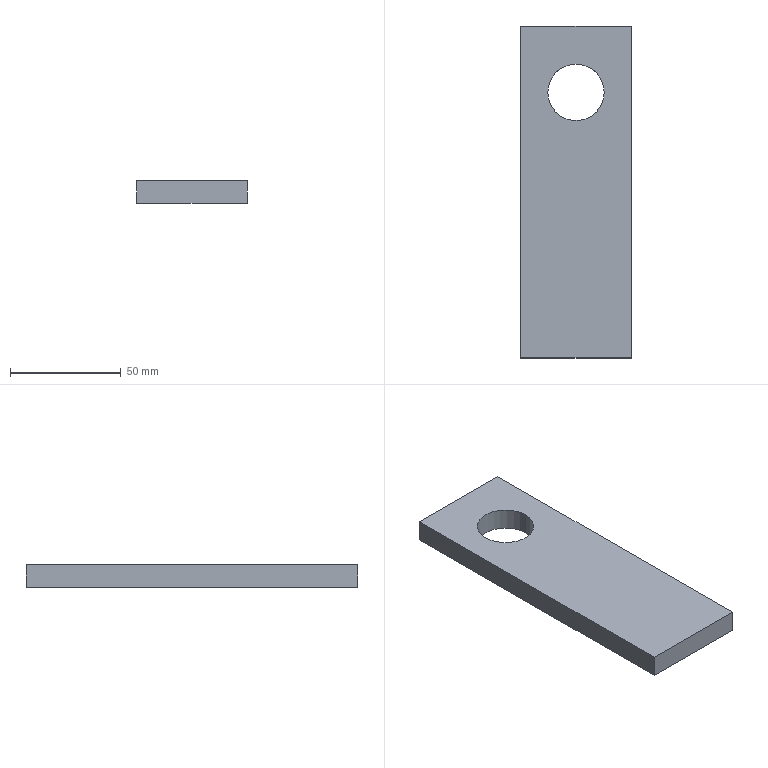Part | SolidWorks | features Extrusion 1, ICE 1 | 1 solid | 8 faces | box 50 x 150 x 10 mm | volume 69893 mm3 | plane 6 | cylinder 2 | commonest cylinder face diameters 25.5 x2
STEP:
#1=CARTESIAN_POINT('',(-12.75,45.,-5.));
#2=VERTEX_POINT('',#1);
#3=CARTESIAN_POINT('',(12.75,45.,-5.));
#4=VERTEX_POINT('',#3);
#5=CARTESIAN_POINT('',(0.,45.,-5.));
#6=DIRECTION('',(0.,0.,1.));
#7=DIRECTION('',(-1.,0.,0.));
#8=AXIS2_PLACEMENT_3D('',#5,#6,#7);
#9=CIRCLE('',#8,12.75);
#10=EDGE_CURVE('',#2,#4,#9,.T.);
#11=ORIENTED_EDGE('',*,*,#10,.F.);
#12=CARTESIAN_POINT('',(-12.75,45.,5.));
#13=VERTEX_POINT('',#12);
#14=CARTESIAN_POINT('',(-12.75,45.,-5.001));
#15=DIRECTION('',(0.,0.,1.));
#16=VECTOR('',#15,1000.);
#17=LINE('',#14,#16);
#18=EDGE_CURVE('',#2,#13,#17,.T.);
#19=ORIENTED_EDGE('',*,*,#18,.T.);
#20=CARTESIAN_POINT('',(12.75,45.,5.));
#21=VERTEX_POINT('',#20);
#22=CARTESIAN_POINT('',(0.,45.,5.));
#23=DIRECTION('',(0.,0.,1.));
#24=DIRECTION('',(1.,0.,0.));
#25=AXIS2_PLACEMENT_3D('',#22,#23,#24);
#26=CIRCLE('',#25,12.75);
#27=EDGE_CURVE('',#13,#21,#26,.T.);
#28=ORIENTED_EDGE('',*,*,#27,.T.);
#29=CARTESIAN_POINT('',(12.75,45.,-5.001));
#30=DIRECTION('',(0.,0.,1.));
#31=VECTOR('',#30,1000.);
#32=LINE('',#29,#31);
#33=EDGE_CURVE('',#4,#21,#32,.T.);
#34=ORIENTED_EDGE('',*,*,#33,.F.);
#35=EDGE_LOOP('',(#11,#19,#28,#34));
#36=FACE_OUTER_BOUND('',#35,.T.);
#37=CARTESIAN_POINT('',(0.,45.,-5.001));
#38=DIRECTION('',(0.,0.,1.));
#39=DIRECTION('',(1.,0.,0.));
#40=AXIS2_PLACEMENT_3D('',#37,#38,#39);
#41=CYLINDRICAL_SURFACE('',#40,12.75);
#42=ADVANCED_FACE('',(#36),#41,.F.);
#43=CARTESIAN_POINT('',(25.,-75.,-5.));
#44=VERTEX_POINT('',#43);
#45=CARTESIAN_POINT('',(25.,75.,-5.));
#46=VERTEX_POINT('',#45);
#47=CARTESIAN_POINT('',(25.,-75.,-5.));
#48=DIRECTION('',(0.,1.,0.));
#49=VECTOR('',#48,1000.);
#50=LINE('',#47,#49);
#51=EDGE_CURVE('',#44,#46,#50,.T.);
#52=ORIENTED_EDGE('',*,*,#51,.T.);
#53=CARTESIAN_POINT('',(25.,75.,5.));
#54=VERTEX_POINT('',#53);
#55=CARTESIAN_POINT('',(25.,75.,5.));
#56=DIRECTION('',(0.,0.,-1.));
#57=VECTOR('',#56,1000.);
#58=LINE('',#55,#57);
#59=EDGE_CURVE('',#54,#46,#58,.T.);
#60=ORIENTED_EDGE('',*,*,#59,.F.);
#61=CARTESIAN_POINT('',(25.,-75.,5.));
#62=VERTEX_POINT('',#61);
#63=CARTESIAN_POINT('',(25.,-75.,5.));
#64=DIRECTION('',(0.,1.,0.));
#65=VECTOR('',#64,1000.);
#66=LINE('',#63,#65);
#67=EDGE_CURVE('',#62,#54,#66,.T.);
#68=ORIENTED_EDGE('',*,*,#67,.F.);
#69=CARTESIAN_POINT('',(25.,-75.,5.));
#70=DIRECTION('',(0.,0.,-1.));
#71=VECTOR('',#70,1000.);
#72=LINE('',#69,#71);
#73=EDGE_CURVE('',#62,#44,#72,.T.);
#74=ORIENTED_EDGE('',*,*,#73,.T.);
#75=EDGE_LOOP('',(#52,#60,#68,#74));
#76=FACE_OUTER_BOUND('',#75,.T.);
#77=CARTESIAN_POINT('',(25.,-75.,5.));
#78=DIRECTION('',(-1.,0.,0.));
#79=DIRECTION('',(0.,0.,1.));
#80=AXIS2_PLACEMENT_3D('',#77,#78,#79);
#81=PLANE('',#80);
#82=ADVANCED_FACE('',(#76),#81,.F.);
#83=CARTESIAN_POINT('',(-25.,75.,-5.));
#84=VERTEX_POINT('',#83);
#85=CARTESIAN_POINT('',(-25.,75.,-5.));
#86=DIRECTION('',(-1.,0.,0.));
#87=VECTOR('',#86,1000.);
#88=LINE('',#85,#87);
#89=EDGE_CURVE('',#46,#84,#88,.T.);
#90=ORIENTED_EDGE('',*,*,#89,.T.);
#91=CARTESIAN_POINT('',(-25.,75.,5.));
#92=VERTEX_POINT('',#91);
#93=CARTESIAN_POINT('',(-25.,75.,5.));
#94=DIRECTION('',(0.,0.,-1.));
#95=VECTOR('',#94,1000.);
#96=LINE('',#93,#95);
#97=EDGE_CURVE('',#92,#84,#96,.T.);
#98=ORIENTED_EDGE('',*,*,#97,.F.);
#99=CARTESIAN_POINT('',(-25.,75.,5.));
#100=DIRECTION('',(-1.,0.,0.));
#101=VECTOR('',#100,1000.);
#102=LINE('',#99,#101);
#103=EDGE_CURVE('',#54,#92,#102,.T.);
#104=ORIENTED_EDGE('',*,*,#103,.F.);
#105=ORIENTED_EDGE('',*,*,#59,.T.);
#106=EDGE_LOOP('',(#90,#98,#104,#105));
#107=FACE_OUTER_BOUND('',#106,.T.);
#108=CARTESIAN_POINT('',(-25.,75.,5.));
#109=DIRECTION('',(0.,-1.,0.));
#110=DIRECTION('',(0.,0.,-1.));
#111=AXIS2_PLACEMENT_3D('',#108,#109,#110);
#112=PLANE('',#111);
#113=ADVANCED_FACE('',(#107),#112,.F.);
#114=CARTESIAN_POINT('',(-25.,-75.,-5.));
#115=VERTEX_POINT('',#114);
#116=CARTESIAN_POINT('',(-25.,-75.,-5.));
#117=DIRECTION('',(0.,-1.,0.));
#118=VECTOR('',#117,1000.);
#119=LINE('',#116,#118);
#120=EDGE_CURVE('',#84,#115,#119,.T.);
#121=ORIENTED_EDGE('',*,*,#120,.T.);
#122=CARTESIAN_POINT('',(-25.,-75.,5.));
#123=VERTEX_POINT('',#122);
#124=CARTESIAN_POINT('',(-25.,-75.,5.));
#125=DIRECTION('',(0.,0.,-1.));
#126=VECTOR('',#125,1000.);
#127=LINE('',#124,#126);
#128=EDGE_CURVE('',#123,#115,#127,.T.);
#129=ORIENTED_EDGE('',*,*,#128,.F.);
#130=CARTESIAN_POINT('',(-25.,-75.,5.));
#131=DIRECTION('',(0.,-1.,0.));
#132=VECTOR('',#131,1000.);
#133=LINE('',#130,#132);
#134=EDGE_CURVE('',#92,#123,#133,.T.);
#135=ORIENTED_EDGE('',*,*,#134,.F.);
#136=ORIENTED_EDGE('',*,*,#97,.T.);
#137=EDGE_LOOP('',(#121,#129,#135,#136));
#138=FACE_OUTER_BOUND('',#137,.T.);
#139=CARTESIAN_POINT('',(-25.,-75.,5.));
#140=DIRECTION('',(1.,0.,0.));
#141=DIRECTION('',(0.,0.,-1.));
#142=AXIS2_PLACEMENT_3D('',#139,#140,#141);
#143=PLANE('',#142);
#144=ADVANCED_FACE('',(#138),#143,.F.);
#145=CARTESIAN_POINT('',(-25.,-75.,-5.));
#146=DIRECTION('',(1.,0.,0.));
#147=VECTOR('',#146,1000.);
#148=LINE('',#145,#147);
#149=EDGE_CURVE('',#115,#44,#148,.T.);
#150=ORIENTED_EDGE('',*,*,#149,.T.);
#151=ORIENTED_EDGE('',*,*,#73,.F.);
#152=CARTESIAN_POINT('',(-25.,-75.,5.));
#153=DIRECTION('',(1.,0.,0.));
#154=VECTOR('',#153,1000.);
#155=LINE('',#152,#154);
#156=EDGE_CURVE('',#123,#62,#155,.T.);
#157=ORIENTED_EDGE('',*,*,#156,.F.);
#158=ORIENTED_EDGE('',*,*,#128,.T.);
#159=EDGE_LOOP('',(#150,#151,#157,#158));
#160=FACE_OUTER_BOUND('',#159,.T.);
#161=CARTESIAN_POINT('',(-25.,-75.,5.));
#162=DIRECTION('',(0.,1.,0.));
#163=DIRECTION('',(0.,0.,1.));
#164=AXIS2_PLACEMENT_3D('',#161,#162,#163);
#165=PLANE('',#164);
#166=ADVANCED_FACE('',(#160),#165,.F.);
#167=CARTESIAN_POINT('',(0.,45.,5.));
#168=DIRECTION('',(0.,0.,1.));
#169=DIRECTION('',(1.,0.,0.));
#170=AXIS2_PLACEMENT_3D('',#167,#168,#169);
#171=CIRCLE('',#170,12.75);
#172=EDGE_CURVE('',#21,#13,#171,.T.);
#173=ORIENTED_EDGE('',*,*,#172,.F.);
#174=ORIENTED_EDGE('',*,*,#27,.F.);
#175=EDGE_LOOP('',(#173,#174));
#176=FACE_BOUND('',#175,.T.);
#177=ORIENTED_EDGE('',*,*,#67,.T.);
#178=ORIENTED_EDGE('',*,*,#103,.T.);
#179=ORIENTED_EDGE('',*,*,#134,.T.);
#180=ORIENTED_EDGE('',*,*,#156,.T.);
#181=EDGE_LOOP('',(#177,#178,#179,#180));
#182=FACE_OUTER_BOUND('',#181,.T.);
#183=CARTESIAN_POINT('',(0.,0.,5.));
#184=DIRECTION('',(0.,0.,-1.));
#185=DIRECTION('',(-1.,0.,0.));
#186=AXIS2_PLACEMENT_3D('',#183,#184,#185);
#187=PLANE('',#186);
#188=ADVANCED_FACE('',(#176,#182),#187,.F.);
#189=CARTESIAN_POINT('',(0.,45.,-5.));
#190=DIRECTION('',(0.,0.,1.));
#191=DIRECTION('',(-1.,0.,0.));
#192=AXIS2_PLACEMENT_3D('',#189,#190,#191);
#193=CIRCLE('',#192,12.75);
#194=EDGE_CURVE('',#4,#2,#193,.T.);
#195=ORIENTED_EDGE('',*,*,#194,.T.);
#196=ORIENTED_EDGE('',*,*,#10,.T.);
#197=EDGE_LOOP('',(#195,#196));
#198=FACE_BOUND('',#197,.T.);
#199=ORIENTED_EDGE('',*,*,#51,.F.);
#200=ORIENTED_EDGE('',*,*,#149,.F.);
#201=ORIENTED_EDGE('',*,*,#120,.F.);
#202=ORIENTED_EDGE('',*,*,#89,.F.);
#203=EDGE_LOOP('',(#199,#200,#201,#202));
#204=FACE_OUTER_BOUND('',#203,.T.);
#205=CARTESIAN_POINT('',(0.,0.,-5.));
#206=DIRECTION('',(0.,0.,-1.));
#207=DIRECTION('',(-1.,0.,0.));
#208=AXIS2_PLACEMENT_3D('',#205,#206,#207);
#209=PLANE('',#208);
#210=ADVANCED_FACE('',(#198,#204),#209,.T.);
#211=ORIENTED_EDGE('',*,*,#18,.F.);
#212=ORIENTED_EDGE('',*,*,#194,.F.);
#213=ORIENTED_EDGE('',*,*,#33,.T.);
#214=ORIENTED_EDGE('',*,*,#172,.T.);
#215=EDGE_LOOP('',(#211,#212,#213,#214));
#216=FACE_OUTER_BOUND('',#215,.T.);
#217=CARTESIAN_POINT('',(0.,45.,-5.001));
#218=DIRECTION('',(0.,0.,1.));
#219=DIRECTION('',(1.,0.,0.));
#220=AXIS2_PLACEMENT_3D('',#217,#218,#219);
#221=CYLINDRICAL_SURFACE('',#220,12.75);
#222=ADVANCED_FACE('',(#216),#221,.F.);
#223=CLOSED_SHELL('',(#42,#82,#113,#144,#166,#188,#210,#222));
#224=MANIFOLD_SOLID_BREP('',#223);
#225=CARTESIAN_POINT('',(0.,0.,0.));
#226=DIRECTION('',(0.,0.,1.));
#227=DIRECTION('',(1.,0.,0.));
#228=AXIS2_PLACEMENT_3D('',#225,#226,#227);
#229=(LENGTH_UNIT()NAMED_UNIT(*)SI_UNIT(.MILLI.,.METRE.));
#230=UNCERTAINTY_MEASURE_WITH_UNIT(LENGTH_MEASURE(0.00001),#229,'','');
#231=(NAMED_UNIT(*)PLANE_ANGLE_UNIT()SI_UNIT($,.RADIAN.));
#232=(NAMED_UNIT(*)SI_UNIT($,.STERADIAN.)SOLID_ANGLE_UNIT());
#233=(GEOMETRIC_REPRESENTATION_CONTEXT(3)GLOBAL_UNCERTAINTY_ASSIGNED_CONTEXT((#230))GLOBAL_UNIT_ASSIGNED_CONTEXT((#229,#231,#232))REPRESENTATION_CONTEXT('',''));
#234=ADVANCED_BREP_SHAPE_REPRESENTATION('',(#224,#228),#233);